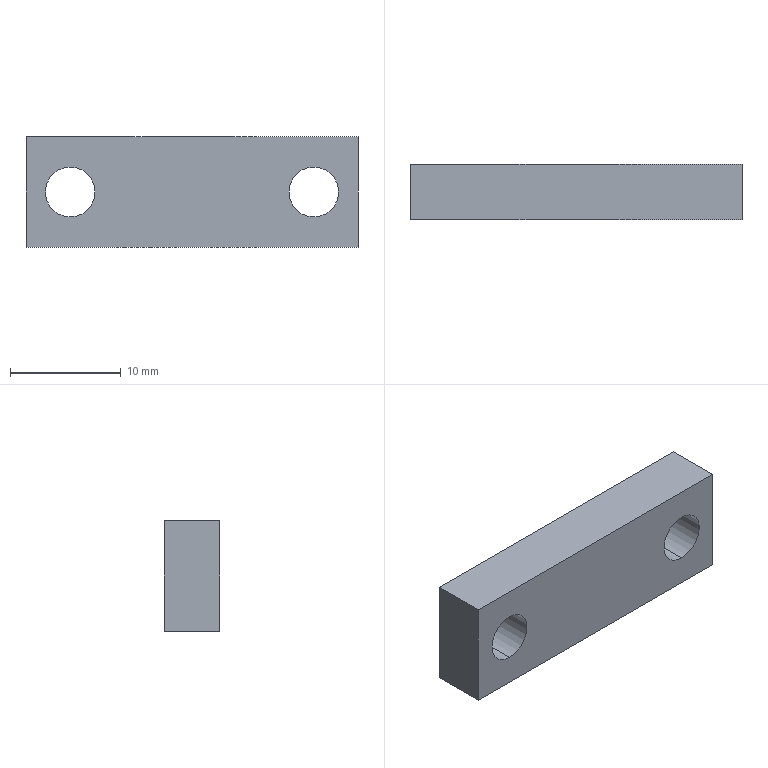Part | SolidWorks | features Extrusion 1, ICE 1 | 1 solid | 10 faces | box 30 x 5 x 10 mm | volume 1341 mm3 | plane 6 | cylinder 4 | commonest cylinder face diameters 4.5 x4
STEP:
#1=CARTESIAN_POINT('',(11.,0.,-2.25));
#2=VERTEX_POINT('',#1);
#3=CARTESIAN_POINT('',(11.,0.,2.25));
#4=VERTEX_POINT('',#3);
#5=CARTESIAN_POINT('',(11.,0.,0.));
#6=DIRECTION('',(0.,1.,0.));
#7=DIRECTION('',(0.,0.,1.));
#8=AXIS2_PLACEMENT_3D('',#5,#6,#7);
#9=CIRCLE('',#8,2.25);
#10=EDGE_CURVE('',#2,#4,#9,.T.);
#11=ORIENTED_EDGE('',*,*,#10,.F.);
#12=CARTESIAN_POINT('',(11.,5.,-2.25));
#13=VERTEX_POINT('',#12);
#14=CARTESIAN_POINT('',(11.,-5.,-2.25));
#15=DIRECTION('',(0.,1.,0.));
#16=VECTOR('',#15,1000.);
#17=LINE('',#14,#16);
#18=EDGE_CURVE('',#2,#13,#17,.T.);
#19=ORIENTED_EDGE('',*,*,#18,.T.);
#20=CARTESIAN_POINT('',(11.,5.,2.25));
#21=VERTEX_POINT('',#20);
#22=CARTESIAN_POINT('',(11.,5.,0.));
#23=DIRECTION('',(0.,1.,0.));
#24=DIRECTION('',(0.,0.,-1.));
#25=AXIS2_PLACEMENT_3D('',#22,#23,#24);
#26=CIRCLE('',#25,2.25);
#27=EDGE_CURVE('',#13,#21,#26,.T.);
#28=ORIENTED_EDGE('',*,*,#27,.T.);
#29=CARTESIAN_POINT('',(11.,-5.,2.25));
#30=DIRECTION('',(0.,1.,0.));
#31=VECTOR('',#30,1000.);
#32=LINE('',#29,#31);
#33=EDGE_CURVE('',#4,#21,#32,.T.);
#34=ORIENTED_EDGE('',*,*,#33,.F.);
#35=EDGE_LOOP('',(#11,#19,#28,#34));
#36=FACE_OUTER_BOUND('',#35,.T.);
#37=CARTESIAN_POINT('',(11.,-5.,0.));
#38=DIRECTION('',(0.,1.,0.));
#39=DIRECTION('',(0.,0.,1.));
#40=AXIS2_PLACEMENT_3D('',#37,#38,#39);
#41=CYLINDRICAL_SURFACE('',#40,2.25);
#42=ADVANCED_FACE('',(#36),#41,.F.);
#43=CARTESIAN_POINT('',(-11.,0.,-2.25));
#44=VERTEX_POINT('',#43);
#45=CARTESIAN_POINT('',(-11.,0.,2.25));
#46=VERTEX_POINT('',#45);
#47=CARTESIAN_POINT('',(-11.,0.,0.));
#48=DIRECTION('',(0.,1.,0.));
#49=DIRECTION('',(0.,0.,1.));
#50=AXIS2_PLACEMENT_3D('',#47,#48,#49);
#51=CIRCLE('',#50,2.25);
#52=EDGE_CURVE('',#44,#46,#51,.T.);
#53=ORIENTED_EDGE('',*,*,#52,.F.);
#54=CARTESIAN_POINT('',(-11.,5.,-2.25));
#55=VERTEX_POINT('',#54);
#56=CARTESIAN_POINT('',(-11.,-5.,-2.25));
#57=DIRECTION('',(0.,1.,0.));
#58=VECTOR('',#57,1000.);
#59=LINE('',#56,#58);
#60=EDGE_CURVE('',#44,#55,#59,.T.);
#61=ORIENTED_EDGE('',*,*,#60,.T.);
#62=CARTESIAN_POINT('',(-11.,5.,2.25));
#63=VERTEX_POINT('',#62);
#64=CARTESIAN_POINT('',(-11.,5.,0.));
#65=DIRECTION('',(0.,1.,0.));
#66=DIRECTION('',(0.,0.,1.));
#67=AXIS2_PLACEMENT_3D('',#64,#65,#66);
#68=CIRCLE('',#67,2.25);
#69=EDGE_CURVE('',#55,#63,#68,.T.);
#70=ORIENTED_EDGE('',*,*,#69,.T.);
#71=CARTESIAN_POINT('',(-11.,-5.,2.25));
#72=DIRECTION('',(0.,1.,0.));
#73=VECTOR('',#72,1000.);
#74=LINE('',#71,#73);
#75=EDGE_CURVE('',#46,#63,#74,.T.);
#76=ORIENTED_EDGE('',*,*,#75,.F.);
#77=EDGE_LOOP('',(#53,#61,#70,#76));
#78=FACE_OUTER_BOUND('',#77,.T.);
#79=CARTESIAN_POINT('',(-11.,-5.,0.));
#80=DIRECTION('',(0.,1.,0.));
#81=DIRECTION('',(0.,0.,1.));
#82=AXIS2_PLACEMENT_3D('',#79,#80,#81);
#83=CYLINDRICAL_SURFACE('',#82,2.25);
#84=ADVANCED_FACE('',(#78),#83,.F.);
#85=CARTESIAN_POINT('',(15.,0.,5.));
#86=VERTEX_POINT('',#85);
#87=CARTESIAN_POINT('',(15.,0.,-5.));
#88=VERTEX_POINT('',#87);
#89=CARTESIAN_POINT('',(15.,0.,-5.));
#90=DIRECTION('',(0.,0.,-1.));
#91=VECTOR('',#90,1000.);
#92=LINE('',#89,#91);
#93=EDGE_CURVE('',#86,#88,#92,.T.);
#94=ORIENTED_EDGE('',*,*,#93,.T.);
#95=CARTESIAN_POINT('',(15.,5.,-5.));
#96=VERTEX_POINT('',#95);
#97=CARTESIAN_POINT('',(15.,5.,-5.));
#98=DIRECTION('',(0.,-1.,0.));
#99=VECTOR('',#98,1000.);
#100=LINE('',#97,#99);
#101=EDGE_CURVE('',#96,#88,#100,.T.);
#102=ORIENTED_EDGE('',*,*,#101,.F.);
#103=CARTESIAN_POINT('',(15.,5.,5.));
#104=VERTEX_POINT('',#103);
#105=CARTESIAN_POINT('',(15.,5.,-5.));
#106=DIRECTION('',(0.,0.,-1.));
#107=VECTOR('',#106,1000.);
#108=LINE('',#105,#107);
#109=EDGE_CURVE('',#104,#96,#108,.T.);
#110=ORIENTED_EDGE('',*,*,#109,.F.);
#111=CARTESIAN_POINT('',(15.,5.,5.));
#112=DIRECTION('',(0.,-1.,0.));
#113=VECTOR('',#112,1000.);
#114=LINE('',#111,#113);
#115=EDGE_CURVE('',#104,#86,#114,.T.);
#116=ORIENTED_EDGE('',*,*,#115,.T.);
#117=EDGE_LOOP('',(#94,#102,#110,#116));
#118=FACE_OUTER_BOUND('',#117,.T.);
#119=CARTESIAN_POINT('',(15.,5.,-5.));
#120=DIRECTION('',(-1.,0.,0.));
#121=DIRECTION('',(0.,0.,1.));
#122=AXIS2_PLACEMENT_3D('',#119,#120,#121);
#123=PLANE('',#122);
#124=ADVANCED_FACE('',(#118),#123,.F.);
#125=CARTESIAN_POINT('',(-15.,0.,-5.));
#126=VERTEX_POINT('',#125);
#127=CARTESIAN_POINT('',(-15.,0.,-5.));
#128=DIRECTION('',(-1.,0.,0.));
#129=VECTOR('',#128,1000.);
#130=LINE('',#127,#129);
#131=EDGE_CURVE('',#88,#126,#130,.T.);
#132=ORIENTED_EDGE('',*,*,#131,.T.);
#133=CARTESIAN_POINT('',(-15.,5.,-5.));
#134=VERTEX_POINT('',#133);
#135=CARTESIAN_POINT('',(-15.,5.,-5.));
#136=DIRECTION('',(0.,-1.,0.));
#137=VECTOR('',#136,1000.);
#138=LINE('',#135,#137);
#139=EDGE_CURVE('',#134,#126,#138,.T.);
#140=ORIENTED_EDGE('',*,*,#139,.F.);
#141=CARTESIAN_POINT('',(-15.,5.,-5.));
#142=DIRECTION('',(-1.,0.,0.));
#143=VECTOR('',#142,1000.);
#144=LINE('',#141,#143);
#145=EDGE_CURVE('',#96,#134,#144,.T.);
#146=ORIENTED_EDGE('',*,*,#145,.F.);
#147=ORIENTED_EDGE('',*,*,#101,.T.);
#148=EDGE_LOOP('',(#132,#140,#146,#147));
#149=FACE_OUTER_BOUND('',#148,.T.);
#150=CARTESIAN_POINT('',(-15.,5.,-5.));
#151=DIRECTION('',(0.,0.,1.));
#152=DIRECTION('',(1.,0.,0.));
#153=AXIS2_PLACEMENT_3D('',#150,#151,#152);
#154=PLANE('',#153);
#155=ADVANCED_FACE('',(#149),#154,.F.);
#156=CARTESIAN_POINT('',(-15.,0.,5.));
#157=VERTEX_POINT('',#156);
#158=CARTESIAN_POINT('',(-15.,0.,-5.));
#159=DIRECTION('',(0.,0.,1.));
#160=VECTOR('',#159,1000.);
#161=LINE('',#158,#160);
#162=EDGE_CURVE('',#126,#157,#161,.T.);
#163=ORIENTED_EDGE('',*,*,#162,.T.);
#164=CARTESIAN_POINT('',(-15.,5.,5.));
#165=VERTEX_POINT('',#164);
#166=CARTESIAN_POINT('',(-15.,5.,5.));
#167=DIRECTION('',(0.,-1.,0.));
#168=VECTOR('',#167,1000.);
#169=LINE('',#166,#168);
#170=EDGE_CURVE('',#165,#157,#169,.T.);
#171=ORIENTED_EDGE('',*,*,#170,.F.);
#172=CARTESIAN_POINT('',(-15.,5.,-5.));
#173=DIRECTION('',(0.,0.,1.));
#174=VECTOR('',#173,1000.);
#175=LINE('',#172,#174);
#176=EDGE_CURVE('',#134,#165,#175,.T.);
#177=ORIENTED_EDGE('',*,*,#176,.F.);
#178=ORIENTED_EDGE('',*,*,#139,.T.);
#179=EDGE_LOOP('',(#163,#171,#177,#178));
#180=FACE_OUTER_BOUND('',#179,.T.);
#181=CARTESIAN_POINT('',(-15.,5.,-5.));
#182=DIRECTION('',(1.,0.,0.));
#183=DIRECTION('',(0.,0.,-1.));
#184=AXIS2_PLACEMENT_3D('',#181,#182,#183);
#185=PLANE('',#184);
#186=ADVANCED_FACE('',(#180),#185,.F.);
#187=CARTESIAN_POINT('',(-15.,0.,5.));
#188=DIRECTION('',(1.,0.,0.));
#189=VECTOR('',#188,1000.);
#190=LINE('',#187,#189);
#191=EDGE_CURVE('',#157,#86,#190,.T.);
#192=ORIENTED_EDGE('',*,*,#191,.T.);
#193=ORIENTED_EDGE('',*,*,#115,.F.);
#194=CARTESIAN_POINT('',(-15.,5.,5.));
#195=DIRECTION('',(1.,0.,0.));
#196=VECTOR('',#195,1000.);
#197=LINE('',#194,#196);
#198=EDGE_CURVE('',#165,#104,#197,.T.);
#199=ORIENTED_EDGE('',*,*,#198,.F.);
#200=ORIENTED_EDGE('',*,*,#170,.T.);
#201=EDGE_LOOP('',(#192,#193,#199,#200));
#202=FACE_OUTER_BOUND('',#201,.T.);
#203=CARTESIAN_POINT('',(-15.,5.,5.));
#204=DIRECTION('',(0.,0.,-1.));
#205=DIRECTION('',(-1.,0.,0.));
#206=AXIS2_PLACEMENT_3D('',#203,#204,#205);
#207=PLANE('',#206);
#208=ADVANCED_FACE('',(#202),#207,.F.);
#209=CARTESIAN_POINT('',(11.,5.,0.));
#210=DIRECTION('',(0.,1.,0.));
#211=DIRECTION('',(0.,0.,-1.));
#212=AXIS2_PLACEMENT_3D('',#209,#210,#211);
#213=CIRCLE('',#212,2.25);
#214=EDGE_CURVE('',#21,#13,#213,.T.);
#215=ORIENTED_EDGE('',*,*,#214,.F.);
#216=ORIENTED_EDGE('',*,*,#27,.F.);
#217=EDGE_LOOP('',(#215,#216));
#218=FACE_BOUND('',#217,.T.);
#219=CARTESIAN_POINT('',(-11.,5.,0.));
#220=DIRECTION('',(0.,1.,0.));
#221=DIRECTION('',(0.,0.,1.));
#222=AXIS2_PLACEMENT_3D('',#219,#220,#221);
#223=CIRCLE('',#222,2.25);
#224=EDGE_CURVE('',#63,#55,#223,.T.);
#225=ORIENTED_EDGE('',*,*,#224,.F.);
#226=ORIENTED_EDGE('',*,*,#69,.F.);
#227=EDGE_LOOP('',(#225,#226));
#228=FACE_BOUND('',#227,.T.);
#229=ORIENTED_EDGE('',*,*,#109,.T.);
#230=ORIENTED_EDGE('',*,*,#145,.T.);
#231=ORIENTED_EDGE('',*,*,#176,.T.);
#232=ORIENTED_EDGE('',*,*,#198,.T.);
#233=EDGE_LOOP('',(#229,#230,#231,#232));
#234=FACE_OUTER_BOUND('',#233,.T.);
#235=CARTESIAN_POINT('',(0.,5.,0.));
#236=DIRECTION('',(0.,1.,0.));
#237=DIRECTION('',(0.,0.,1.));
#238=AXIS2_PLACEMENT_3D('',#235,#236,#237);
#239=PLANE('',#238);
#240=ADVANCED_FACE('',(#218,#228,#234),#239,.T.);
#241=CARTESIAN_POINT('',(11.,0.,0.));
#242=DIRECTION('',(0.,1.,0.));
#243=DIRECTION('',(0.,0.,1.));
#244=AXIS2_PLACEMENT_3D('',#241,#242,#243);
#245=CIRCLE('',#244,2.25);
#246=EDGE_CURVE('',#4,#2,#245,.T.);
#247=ORIENTED_EDGE('',*,*,#246,.T.);
#248=ORIENTED_EDGE('',*,*,#10,.T.);
#249=EDGE_LOOP('',(#247,#248));
#250=FACE_BOUND('',#249,.T.);
#251=CARTESIAN_POINT('',(-11.,0.,0.));
#252=DIRECTION('',(0.,1.,0.));
#253=DIRECTION('',(0.,0.,1.));
#254=AXIS2_PLACEMENT_3D('',#251,#252,#253);
#255=CIRCLE('',#254,2.25);
#256=EDGE_CURVE('',#46,#44,#255,.T.);
#257=ORIENTED_EDGE('',*,*,#256,.T.);
#258=ORIENTED_EDGE('',*,*,#52,.T.);
#259=EDGE_LOOP('',(#257,#258));
#260=FACE_BOUND('',#259,.T.);
#261=ORIENTED_EDGE('',*,*,#93,.F.);
#262=ORIENTED_EDGE('',*,*,#191,.F.);
#263=ORIENTED_EDGE('',*,*,#162,.F.);
#264=ORIENTED_EDGE('',*,*,#131,.F.);
#265=EDGE_LOOP('',(#261,#262,#263,#264));
#266=FACE_OUTER_BOUND('',#265,.T.);
#267=CARTESIAN_POINT('',(0.,0.,0.));
#268=DIRECTION('',(0.,1.,0.));
#269=DIRECTION('',(0.,0.,1.));
#270=AXIS2_PLACEMENT_3D('',#267,#268,#269);
#271=PLANE('',#270);
#272=ADVANCED_FACE('',(#250,#260,#266),#271,.F.);
#273=ORIENTED_EDGE('',*,*,#60,.F.);
#274=ORIENTED_EDGE('',*,*,#256,.F.);
#275=ORIENTED_EDGE('',*,*,#75,.T.);
#276=ORIENTED_EDGE('',*,*,#224,.T.);
#277=EDGE_LOOP('',(#273,#274,#275,#276));
#278=FACE_OUTER_BOUND('',#277,.T.);
#279=CARTESIAN_POINT('',(-11.,-5.,0.));
#280=DIRECTION('',(0.,1.,0.));
#281=DIRECTION('',(0.,0.,1.));
#282=AXIS2_PLACEMENT_3D('',#279,#280,#281);
#283=CYLINDRICAL_SURFACE('',#282,2.25);
#284=ADVANCED_FACE('',(#278),#283,.F.);
#285=ORIENTED_EDGE('',*,*,#18,.F.);
#286=ORIENTED_EDGE('',*,*,#246,.F.);
#287=ORIENTED_EDGE('',*,*,#33,.T.);
#288=ORIENTED_EDGE('',*,*,#214,.T.);
#289=EDGE_LOOP('',(#285,#286,#287,#288));
#290=FACE_OUTER_BOUND('',#289,.T.);
#291=CARTESIAN_POINT('',(11.,-5.,0.));
#292=DIRECTION('',(0.,1.,0.));
#293=DIRECTION('',(0.,0.,1.));
#294=AXIS2_PLACEMENT_3D('',#291,#292,#293);
#295=CYLINDRICAL_SURFACE('',#294,2.25);
#296=ADVANCED_FACE('',(#290),#295,.F.);
#297=CLOSED_SHELL('',(#42,#84,#124,#155,#186,#208,#240,#272,#284,#296));
#298=MANIFOLD_SOLID_BREP('',#297);
#299=CARTESIAN_POINT('',(0.,0.,0.));
#300=DIRECTION('',(0.,0.,1.));
#301=DIRECTION('',(1.,0.,0.));
#302=AXIS2_PLACEMENT_3D('',#299,#300,#301);
#303=(LENGTH_UNIT()NAMED_UNIT(*)SI_UNIT(.MILLI.,.METRE.));
#304=UNCERTAINTY_MEASURE_WITH_UNIT(LENGTH_MEASURE(0.00001),#303,'','');
#305=(NAMED_UNIT(*)PLANE_ANGLE_UNIT()SI_UNIT($,.RADIAN.));
#306=(NAMED_UNIT(*)SI_UNIT($,.STERADIAN.)SOLID_ANGLE_UNIT());
#307=(GEOMETRIC_REPRESENTATION_CONTEXT(3)GLOBAL_UNCERTAINTY_ASSIGNED_CONTEXT((#304))GLOBAL_UNIT_ASSIGNED_CONTEXT((#303,#305,#306))REPRESENTATION_CONTEXT('',''));
#308=ADVANCED_BREP_SHAPE_REPRESENTATION('',(#298,#302),#307);